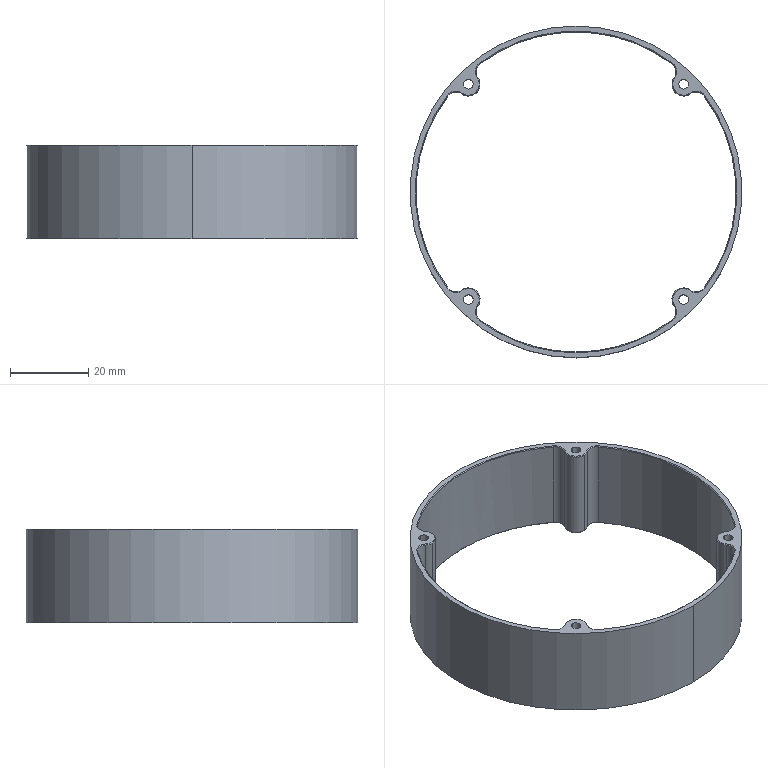NC program | NX | posted with a generic post | part box 85 x 85 x 24 mm
Lines 6746 to 6793 of 6793:
(刀补 , TOOL : D10JING)
N13454 T14 M6
N13456 G54
N13458 G17 G0 G90 X-28.947 Y17.572 S9500 M3
N13460 G43 Z30. H14
N13462 Z-11.
N13464 G94 G1 Z-12. F1000.
N13466 G41 X-28.951 Y17.672 D14
N13468 X-29.294 Y19.207
N13470 G3 X-29.971 Y19.944 R1.
N13472 X-29.971 Y-19.944 R36. F1200.
N13474 G2 X-19.944 Y-29.971 R8.
N13476 G3 X19.944 Y-29.971 R36.
N13478 G2 X29.971 Y-19.944 R8.
N13480 G3 X29.971 Y19.944 R36.
N13482 G2 X19.944 Y29.971 R8.
N13484 G3 X-19.944 Y29.971 R36.
N13486 G2 X-29.971 Y19.944 R8.
N13488 G3 X-30.005 Y18.944 R1.
N13490 G1 X-29.196 Y17.424
N13492 G40
N13494 X-29.134 Y17.345
N13496 Z-11.
N13498 G0 Z30.
N13500 X-28.947 Y17.572
N13502 Z-23.
N13504 G1 Z-24. F1000.
N13506 G41 X-28.951 Y17.672
N13508 X-29.294 Y19.207
N13510 G3 X-29.971 Y19.944 R1.
N13512 X-29.971 Y-19.944 R36. F1200.
N13514 G2 X-19.944 Y-29.971 R8.
N13516 G3 X19.944 Y-29.971 R36.
N13518 G2 X29.971 Y-19.944 R8.
N13520 G3 X29.971 Y19.944 R36.
N13522 G2 X19.944 Y29.971 R8.
N13524 G3 X-19.944 Y29.971 R36.
N13526 G2 X-29.971 Y19.944 R8.
N13528 G3 X-30.005 Y18.944 R1.
N13530 G1 X-29.196 Y17.424
N13532 G40
N13534 X-29.134 Y17.345
N13536 Z-23.
N13538 G0 Z30.
N13540 M5
N13542 M2